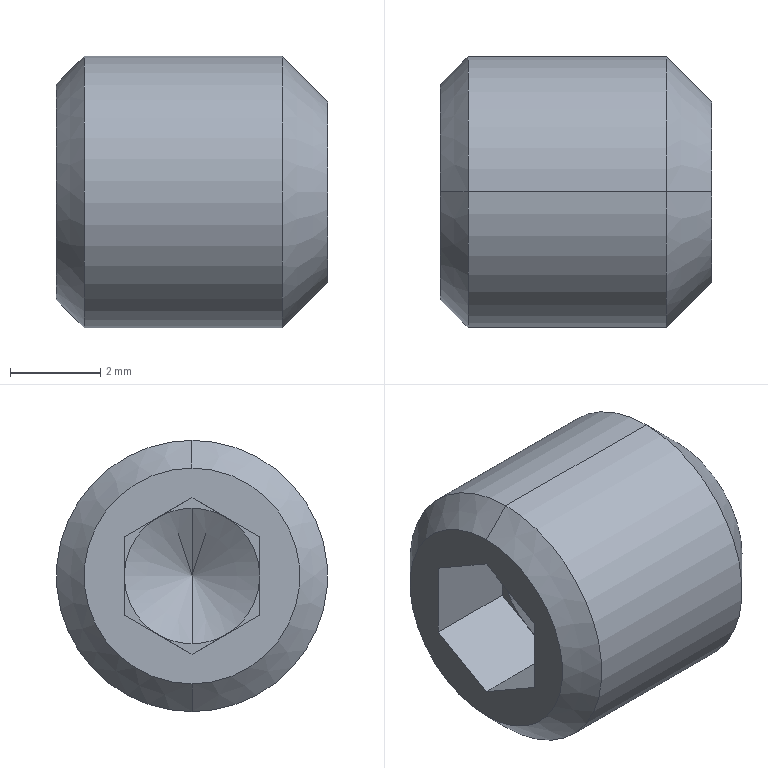Part | SolidWorks | features BaseBody 1 | 1 solid | 22 faces | box 6 x 6 x 6 mm | volume 140.334 mm3 | plane 14 | cone 6 | cylinder 2 | commonest cylinder face diameters 6 x2
STEP:
#1=CARTESIAN_POINT('',(-1.,0.,3.));
#2=VERTEX_POINT('',#1);
#3=CARTESIAN_POINT('',(-1.,0.,-3.));
#4=VERTEX_POINT('',#3);
#5=CARTESIAN_POINT('',(-1.,0.,0.));
#6=DIRECTION('',(-1.,0.,0.));
#7=DIRECTION('',(0.,0.,1.));
#8=AXIS2_PLACEMENT_3D('',#5,#6,#7);
#9=CIRCLE('',#8,3.);
#10=EDGE_CURVE('',#2,#4,#9,.T.);
#11=ORIENTED_EDGE('',*,*,#10,.T.);
#12=CARTESIAN_POINT('',(-5.386,0.,-3.));
#13=VERTEX_POINT('',#12);
#14=CARTESIAN_POINT('',(0.,0.,-3.));
#15=DIRECTION('',(-1.,0.,0.));
#16=VECTOR('',#15,1000.);
#17=LINE('',#14,#16);
#18=EDGE_CURVE('',#4,#13,#17,.T.);
#19=ORIENTED_EDGE('',*,*,#18,.T.);
#20=CARTESIAN_POINT('',(-5.386,0.,3.));
#21=VERTEX_POINT('',#20);
#22=CARTESIAN_POINT('',(-5.386,0.,0.));
#23=DIRECTION('',(1.,0.,0.));
#24=DIRECTION('',(0.,0.,1.));
#25=AXIS2_PLACEMENT_3D('',#22,#23,#24);
#26=CIRCLE('',#25,3.);
#27=EDGE_CURVE('',#13,#21,#26,.T.);
#28=ORIENTED_EDGE('',*,*,#27,.T.);
#29=CARTESIAN_POINT('',(0.,0.,3.));
#30=DIRECTION('',(-1.,0.,0.));
#31=VECTOR('',#30,1000.);
#32=LINE('',#29,#31);
#33=EDGE_CURVE('',#2,#21,#32,.T.);
#34=ORIENTED_EDGE('',*,*,#33,.F.);
#35=EDGE_LOOP('',(#11,#19,#28,#34));
#36=FACE_OUTER_BOUND('',#35,.T.);
#37=CARTESIAN_POINT('',(0.,0.,0.));
#38=DIRECTION('',(-1.,0.,0.));
#39=DIRECTION('',(0.,0.,1.));
#40=AXIS2_PLACEMENT_3D('',#37,#38,#39);
#41=CYLINDRICAL_SURFACE('',#40,3.);
#42=ADVANCED_FACE('',(#36),#41,.T.);
#43=CARTESIAN_POINT('',(-6.,0.,-2.387));
#44=VERTEX_POINT('',#43);
#45=CARTESIAN_POINT('',(-6.,0.,2.387));
#46=VERTEX_POINT('',#45);
#47=CARTESIAN_POINT('',(-6.,0.,0.));
#48=DIRECTION('',(1.,0.,0.));
#49=DIRECTION('',(0.,0.,-1.));
#50=AXIS2_PLACEMENT_3D('',#47,#48,#49);
#51=CIRCLE('',#50,2.387);
#52=EDGE_CURVE('',#44,#46,#51,.T.);
#53=ORIENTED_EDGE('',*,*,#52,.T.);
#54=CARTESIAN_POINT('',(-5.386,0.,3.));
#55=DIRECTION('',(0.7071,0.,0.7071));
#56=VECTOR('',#55,1000.);
#57=LINE('',#54,#56);
#58=EDGE_CURVE('',#46,#21,#57,.T.);
#59=ORIENTED_EDGE('',*,*,#58,.T.);
#60=ORIENTED_EDGE('',*,*,#27,.F.);
#61=CARTESIAN_POINT('',(-5.386,0.,-3.));
#62=DIRECTION('',(0.7071,0.,-0.7071));
#63=VECTOR('',#62,1000.);
#64=LINE('',#61,#63);
#65=EDGE_CURVE('',#44,#13,#64,.T.);
#66=ORIENTED_EDGE('',*,*,#65,.F.);
#67=EDGE_LOOP('',(#53,#59,#60,#66));
#68=FACE_OUTER_BOUND('',#67,.T.);
#69=CARTESIAN_POINT('',(-5.386,0.,0.));
#70=DIRECTION('',(1.,0.,0.));
#71=DIRECTION('',(0.,0.,-1.));
#72=AXIS2_PLACEMENT_3D('',#69,#70,#71);
#73=CONICAL_SURFACE('',#72,3.,0.7854);
#74=ADVANCED_FACE('',(#68),#73,.T.);
#75=CARTESIAN_POINT('',(0.,0.,2.));
#76=VERTEX_POINT('',#75);
#77=CARTESIAN_POINT('',(0.,0.,-2.));
#78=VERTEX_POINT('',#77);
#79=CARTESIAN_POINT('',(0.,0.,0.));
#80=DIRECTION('',(-1.,0.,0.));
#81=DIRECTION('',(0.,0.,1.));
#82=AXIS2_PLACEMENT_3D('',#79,#80,#81);
#83=CIRCLE('',#82,2.);
#84=EDGE_CURVE('',#76,#78,#83,.T.);
#85=ORIENTED_EDGE('',*,*,#84,.T.);
#86=CARTESIAN_POINT('',(-1.,0.,-3.));
#87=DIRECTION('',(-0.7071,0.,-0.7071));
#88=VECTOR('',#87,1000.);
#89=LINE('',#86,#88);
#90=EDGE_CURVE('',#78,#4,#89,.T.);
#91=ORIENTED_EDGE('',*,*,#90,.T.);
#92=ORIENTED_EDGE('',*,*,#10,.F.);
#93=CARTESIAN_POINT('',(-1.,0.,3.));
#94=DIRECTION('',(-0.7071,0.,0.7071));
#95=VECTOR('',#94,1000.);
#96=LINE('',#93,#95);
#97=EDGE_CURVE('',#76,#2,#96,.T.);
#98=ORIENTED_EDGE('',*,*,#97,.F.);
#99=EDGE_LOOP('',(#85,#91,#92,#98));
#100=FACE_OUTER_BOUND('',#99,.T.);
#101=CARTESIAN_POINT('',(-1.,0.,0.));
#102=DIRECTION('',(-1.,0.,0.));
#103=DIRECTION('',(0.,0.,1.));
#104=AXIS2_PLACEMENT_3D('',#101,#102,#103);
#105=CONICAL_SURFACE('',#104,3.,0.7854);
#106=ADVANCED_FACE('',(#100),#105,.T.);
#107=CARTESIAN_POINT('',(-3.134,0.,0.));
#108=VERTEX_POINT('',#107);
#109=CARTESIAN_POINT('',(-4.,0.,1.5));
#110=VERTEX_POINT('',#109);
#111=CARTESIAN_POINT('',(-4.,0.,1.5));
#112=DIRECTION('',(-0.5,0.,0.866));
#113=VECTOR('',#112,1000.);
#114=LINE('',#111,#113);
#115=EDGE_CURVE('',#108,#110,#114,.T.);
#116=ORIENTED_EDGE('',*,*,#115,.F.);
#117=CARTESIAN_POINT('',(-4.,0.,-1.5));
#118=VERTEX_POINT('',#117);
#119=CARTESIAN_POINT('',(-4.,0.,-1.5));
#120=DIRECTION('',(-0.5,0.,-0.866));
#121=VECTOR('',#120,1000.);
#122=LINE('',#119,#121);
#123=EDGE_CURVE('',#108,#118,#122,.T.);
#124=ORIENTED_EDGE('',*,*,#123,.T.);
#125=CARTESIAN_POINT('',(-4.,-0.75,-1.299));
#126=VERTEX_POINT('',#125);
#127=CARTESIAN_POINT('',(-4.,0.,0.));
#128=DIRECTION('',(1.,0.,0.));
#129=DIRECTION('',(0.,0.,1.));
#130=AXIS2_PLACEMENT_3D('',#127,#128,#129);
#131=CIRCLE('',#130,1.5);
#132=EDGE_CURVE('',#126,#118,#131,.T.);
#133=ORIENTED_EDGE('',*,*,#132,.F.);
#134=CARTESIAN_POINT('',(-4.,-1.5,0.));
#135=VERTEX_POINT('',#134);
#136=CARTESIAN_POINT('',(-4.,0.,0.));
#137=DIRECTION('',(1.,0.,0.));
#138=DIRECTION('',(0.,0.,1.));
#139=AXIS2_PLACEMENT_3D('',#136,#137,#138);
#140=CIRCLE('',#139,1.5);
#141=EDGE_CURVE('',#135,#126,#140,.T.);
#142=ORIENTED_EDGE('',*,*,#141,.F.);
#143=CARTESIAN_POINT('',(-4.,-0.75,1.299));
#144=VERTEX_POINT('',#143);
#145=CARTESIAN_POINT('',(-4.,0.,0.));
#146=DIRECTION('',(1.,0.,0.));
#147=DIRECTION('',(0.,0.,1.));
#148=AXIS2_PLACEMENT_3D('',#145,#146,#147);
#149=CIRCLE('',#148,1.5);
#150=EDGE_CURVE('',#144,#135,#149,.T.);
#151=ORIENTED_EDGE('',*,*,#150,.F.);
#152=CARTESIAN_POINT('',(-4.,0.,0.));
#153=DIRECTION('',(1.,0.,0.));
#154=DIRECTION('',(0.,0.,1.));
#155=AXIS2_PLACEMENT_3D('',#152,#153,#154);
#156=CIRCLE('',#155,1.5);
#157=EDGE_CURVE('',#110,#144,#156,.T.);
#158=ORIENTED_EDGE('',*,*,#157,.F.);
#159=EDGE_LOOP('',(#116,#124,#133,#142,#151,#158));
#160=FACE_OUTER_BOUND('',#159,.T.);
#161=CARTESIAN_POINT('',(-4.,0.,0.));
#162=DIRECTION('',(-1.,0.,0.));
#163=DIRECTION('',(0.,0.,1.));
#164=AXIS2_PLACEMENT_3D('',#161,#162,#163);
#165=CONICAL_SURFACE('',#164,1.5,1.047);
#166=ADVANCED_FACE('',(#160),#165,.F.);
#167=ORIENTED_EDGE('',*,*,#18,.F.);
#168=CARTESIAN_POINT('',(-1.,0.,0.));
#169=DIRECTION('',(-1.,0.,0.));
#170=DIRECTION('',(0.,0.,1.));
#171=AXIS2_PLACEMENT_3D('',#168,#169,#170);
#172=CIRCLE('',#171,3.);
#173=EDGE_CURVE('',#4,#2,#172,.T.);
#174=ORIENTED_EDGE('',*,*,#173,.T.);
#175=ORIENTED_EDGE('',*,*,#33,.T.);
#176=CARTESIAN_POINT('',(-5.386,0.,0.));
#177=DIRECTION('',(1.,0.,0.));
#178=DIRECTION('',(0.,0.,1.));
#179=AXIS2_PLACEMENT_3D('',#176,#177,#178);
#180=CIRCLE('',#179,3.);
#181=EDGE_CURVE('',#21,#13,#180,.T.);
#182=ORIENTED_EDGE('',*,*,#181,.T.);
#183=EDGE_LOOP('',(#167,#174,#175,#182));
#184=FACE_OUTER_BOUND('',#183,.T.);
#185=CARTESIAN_POINT('',(0.,0.,0.));
#186=DIRECTION('',(-1.,0.,0.));
#187=DIRECTION('',(0.,0.,1.));
#188=AXIS2_PLACEMENT_3D('',#185,#186,#187);
#189=CYLINDRICAL_SURFACE('',#188,3.);
#190=ADVANCED_FACE('',(#184),#189,.T.);
#191=ORIENTED_EDGE('',*,*,#58,.F.);
#192=CARTESIAN_POINT('',(-6.,0.,0.));
#193=DIRECTION('',(1.,0.,0.));
#194=DIRECTION('',(0.,0.,-1.));
#195=AXIS2_PLACEMENT_3D('',#192,#193,#194);
#196=CIRCLE('',#195,2.387);
#197=EDGE_CURVE('',#46,#44,#196,.T.);
#198=ORIENTED_EDGE('',*,*,#197,.T.);
#199=ORIENTED_EDGE('',*,*,#65,.T.);
#200=ORIENTED_EDGE('',*,*,#181,.F.);
#201=EDGE_LOOP('',(#191,#198,#199,#200));
#202=FACE_OUTER_BOUND('',#201,.T.);
#203=CARTESIAN_POINT('',(-5.386,0.,0.));
#204=DIRECTION('',(1.,0.,0.));
#205=DIRECTION('',(0.,0.,-1.));
#206=AXIS2_PLACEMENT_3D('',#203,#204,#205);
#207=CONICAL_SURFACE('',#206,3.,0.7854);
#208=ADVANCED_FACE('',(#202),#207,.T.);
#209=ORIENTED_EDGE('',*,*,#90,.F.);
#210=CARTESIAN_POINT('',(0.,0.,0.));
#211=DIRECTION('',(-1.,0.,0.));
#212=DIRECTION('',(0.,0.,1.));
#213=AXIS2_PLACEMENT_3D('',#210,#211,#212);
#214=CIRCLE('',#213,2.);
#215=EDGE_CURVE('',#78,#76,#214,.T.);
#216=ORIENTED_EDGE('',*,*,#215,.T.);
#217=ORIENTED_EDGE('',*,*,#97,.T.);
#218=ORIENTED_EDGE('',*,*,#173,.F.);
#219=EDGE_LOOP('',(#209,#216,#217,#218));
#220=FACE_OUTER_BOUND('',#219,.T.);
#221=CARTESIAN_POINT('',(-1.,0.,0.));
#222=DIRECTION('',(-1.,0.,0.));
#223=DIRECTION('',(0.,0.,1.));
#224=AXIS2_PLACEMENT_3D('',#221,#222,#223);
#225=CONICAL_SURFACE('',#224,3.,0.7854);
#226=ADVANCED_FACE('',(#220),#225,.T.);
#227=CARTESIAN_POINT('',(-6.,0.,1.732));
#228=VERTEX_POINT('',#227);
#229=CARTESIAN_POINT('',(-6.,-1.5,0.866));
#230=VERTEX_POINT('',#229);
#231=CARTESIAN_POINT('',(-6.,-1.5,0.866));
#232=DIRECTION('',(0.,-0.866,-0.5));
#233=VECTOR('',#232,1000.);
#234=LINE('',#231,#233);
#235=EDGE_CURVE('',#228,#230,#234,.T.);
#236=ORIENTED_EDGE('',*,*,#235,.T.);
#237=CARTESIAN_POINT('',(-6.,-1.5,-0.866));
#238=VERTEX_POINT('',#237);
#239=CARTESIAN_POINT('',(-6.,-1.5,-0.866));
#240=DIRECTION('',(0.,0.,-1.));
#241=VECTOR('',#240,1000.);
#242=LINE('',#239,#241);
#243=EDGE_CURVE('',#230,#238,#242,.T.);
#244=ORIENTED_EDGE('',*,*,#243,.T.);
#245=CARTESIAN_POINT('',(-6.,0.,-1.732));
#246=VERTEX_POINT('',#245);
#247=CARTESIAN_POINT('',(-6.,0.,-1.732));
#248=DIRECTION('',(0.,0.866,-0.5));
#249=VECTOR('',#248,1000.);
#250=LINE('',#247,#249);
#251=EDGE_CURVE('',#238,#246,#250,.T.);
#252=ORIENTED_EDGE('',*,*,#251,.T.);
#253=CARTESIAN_POINT('',(-6.,1.5,-0.866));
#254=VERTEX_POINT('',#253);
#255=CARTESIAN_POINT('',(-6.,1.5,-0.866));
#256=DIRECTION('',(0.,0.866,0.5));
#257=VECTOR('',#256,1000.);
#258=LINE('',#255,#257);
#259=EDGE_CURVE('',#246,#254,#258,.T.);
#260=ORIENTED_EDGE('',*,*,#259,.T.);
#261=CARTESIAN_POINT('',(-6.,1.5,0.866));
#262=VERTEX_POINT('',#261);
#263=CARTESIAN_POINT('',(-6.,1.5,0.866));
#264=DIRECTION('',(0.,0.,1.));
#265=VECTOR('',#264,1000.);
#266=LINE('',#263,#265);
#267=EDGE_CURVE('',#254,#262,#266,.T.);
#268=ORIENTED_EDGE('',*,*,#267,.T.);
#269=CARTESIAN_POINT('',(-6.,0.,1.732));
#270=DIRECTION('',(0.,0.866,-0.5));
#271=VECTOR('',#270,1000.);
#272=LINE('',#269,#271);
#273=EDGE_CURVE('',#228,#262,#272,.T.);
#274=ORIENTED_EDGE('',*,*,#273,.F.);
#275=EDGE_LOOP('',(#236,#244,#252,#260,#268,#274));
#276=FACE_BOUND('',#275,.T.);
#277=ORIENTED_EDGE('',*,*,#52,.F.);
#278=ORIENTED_EDGE('',*,*,#197,.F.);
#279=EDGE_LOOP('',(#277,#278));
#280=FACE_OUTER_BOUND('',#279,.T.);
#281=CARTESIAN_POINT('',(-6.,0.,0.));
#282=DIRECTION('',(1.,0.,0.));
#283=DIRECTION('',(0.,0.,-1.));
#284=AXIS2_PLACEMENT_3D('',#281,#282,#283);
#285=PLANE('',#284);
#286=ADVANCED_FACE('',(#276,#280),#285,.F.);
#287=ORIENTED_EDGE('',*,*,#84,.F.);
#288=ORIENTED_EDGE('',*,*,#215,.F.);
#289=EDGE_LOOP('',(#287,#288));
#290=FACE_OUTER_BOUND('',#289,.T.);
#291=CARTESIAN_POINT('',(0.,2.,0.));
#292=DIRECTION('',(-1.,0.,0.));
#293=DIRECTION('',(0.,0.,1.));
#294=AXIS2_PLACEMENT_3D('',#291,#292,#293);
#295=PLANE('',#294);
#296=ADVANCED_FACE('',(#290),#295,.F.);
#297=CARTESIAN_POINT('',(-4.,1.5,0.866));
#298=VERTEX_POINT('',#297);
#299=CARTESIAN_POINT('',(-4.,1.5,0.866));
#300=DIRECTION('',(-1.,0.,0.));
#301=VECTOR('',#300,1000.);
#302=LINE('',#299,#301);
#303=EDGE_CURVE('',#298,#262,#302,.T.);
#304=ORIENTED_EDGE('',*,*,#303,.F.);
#305=CARTESIAN_POINT('',(-4.,0.75,1.299));
#306=VERTEX_POINT('',#305);
#307=CARTESIAN_POINT('',(-4.,0.,1.732));
#308=DIRECTION('',(0.,0.866,-0.5));
#309=VECTOR('',#308,1000.);
#310=LINE('',#307,#309);
#311=EDGE_CURVE('',#306,#298,#310,.T.);
#312=ORIENTED_EDGE('',*,*,#311,.F.);
#313=CARTESIAN_POINT('',(-4.,0.,1.732));
#314=VERTEX_POINT('',#313);
#315=CARTESIAN_POINT('',(-4.,0.,1.732));
#316=DIRECTION('',(0.,0.866,-0.5));
#317=VECTOR('',#316,1000.);
#318=LINE('',#315,#317);
#319=EDGE_CURVE('',#314,#306,#318,.T.);
#320=ORIENTED_EDGE('',*,*,#319,.F.);
#321=CARTESIAN_POINT('',(-4.,0.,1.732));
#322=DIRECTION('',(1.,0.,0.));
#323=VECTOR('',#322,1000.);
#324=LINE('',#321,#323);
#325=EDGE_CURVE('',#228,#314,#324,.T.);
#326=ORIENTED_EDGE('',*,*,#325,.F.);
#327=ORIENTED_EDGE('',*,*,#273,.T.);
#328=EDGE_LOOP('',(#304,#312,#320,#326,#327));
#329=FACE_OUTER_BOUND('',#328,.T.);
#330=CARTESIAN_POINT('',(-4.,0.,1.732));
#331=DIRECTION('',(0.,0.5,0.866));
#332=DIRECTION('',(0.,-0.866,0.5));
#333=AXIS2_PLACEMENT_3D('',#330,#331,#332);
#334=PLANE('',#333);
#335=ADVANCED_FACE('',(#329),#334,.F.);
#336=ORIENTED_EDGE('',*,*,#267,.F.);
#337=CARTESIAN_POINT('',(-4.,1.5,-0.866));
#338=VERTEX_POINT('',#337);
#339=CARTESIAN_POINT('',(-4.,1.5,-0.866));
#340=DIRECTION('',(-1.,0.,0.));
#341=VECTOR('',#340,1000.);
#342=LINE('',#339,#341);
#343=EDGE_CURVE('',#338,#254,#342,.T.);
#344=ORIENTED_EDGE('',*,*,#343,.F.);
#345=CARTESIAN_POINT('',(-4.,1.5,0.));
#346=VERTEX_POINT('',#345);
#347=CARTESIAN_POINT('',(-4.,1.5,0.866));
#348=DIRECTION('',(0.,0.,-1.));
#349=VECTOR('',#348,1000.);
#350=LINE('',#347,#349);
#351=EDGE_CURVE('',#346,#338,#350,.T.);
#352=ORIENTED_EDGE('',*,*,#351,.F.);
#353=CARTESIAN_POINT('',(-4.,1.5,0.866));
#354=DIRECTION('',(0.,0.,-1.));
#355=VECTOR('',#354,1000.);
#356=LINE('',#353,#355);
#357=EDGE_CURVE('',#298,#346,#356,.T.);
#358=ORIENTED_EDGE('',*,*,#357,.F.);
#359=ORIENTED_EDGE('',*,*,#303,.T.);
#360=EDGE_LOOP('',(#336,#344,#352,#358,#359));
#361=FACE_OUTER_BOUND('',#360,.T.);
#362=CARTESIAN_POINT('',(-4.,1.5,0.866));
#363=DIRECTION('',(0.,1.,0.));
#364=DIRECTION('',(0.,0.,1.));
#365=AXIS2_PLACEMENT_3D('',#362,#363,#364);
#366=PLANE('',#365);
#367=ADVANCED_FACE('',(#361),#366,.F.);
#368=CARTESIAN_POINT('',(-4.,0.,0.));
#369=DIRECTION('',(1.,0.,0.));
#370=DIRECTION('',(0.,0.,1.));
#371=AXIS2_PLACEMENT_3D('',#368,#369,#370);
#372=CIRCLE('',#371,1.5);
#373=EDGE_CURVE('',#346,#306,#372,.T.);
#374=ORIENTED_EDGE('',*,*,#373,.T.);
#375=ORIENTED_EDGE('',*,*,#311,.T.);
#376=ORIENTED_EDGE('',*,*,#357,.T.);
#377=EDGE_LOOP('',(#374,#375,#376));
#378=FACE_OUTER_BOUND('',#377,.T.);
#379=CARTESIAN_POINT('',(-4.,0.,0.));
#380=DIRECTION('',(-1.,0.,0.));
#381=DIRECTION('',(0.,0.,1.));
#382=AXIS2_PLACEMENT_3D('',#379,#380,#381);
#383=PLANE('',#382);
#384=ADVANCED_FACE('',(#378),#383,.T.);
#385=CARTESIAN_POINT('',(-4.,0.,0.));
#386=DIRECTION('',(1.,0.,0.));
#387=DIRECTION('',(0.,0.,1.));
#388=AXIS2_PLACEMENT_3D('',#385,#386,#387);
#389=CIRCLE('',#388,1.5);
#390=EDGE_CURVE('',#306,#110,#389,.T.);
#391=ORIENTED_EDGE('',*,*,#390,.T.);
#392=ORIENTED_EDGE('',*,*,#157,.T.);
#393=CARTESIAN_POINT('',(-4.,-0.75,1.299));
#394=DIRECTION('',(0.,0.866,0.5));
#395=VECTOR('',#394,1000.);
#396=LINE('',#393,#395);
#397=EDGE_CURVE('',#144,#314,#396,.T.);
#398=ORIENTED_EDGE('',*,*,#397,.T.);
#399=ORIENTED_EDGE('',*,*,#319,.T.);
#400=EDGE_LOOP('',(#391,#392,#398,#399));
#401=FACE_OUTER_BOUND('',#400,.T.);
#402=CARTESIAN_POINT('',(-4.,0.,0.));
#403=DIRECTION('',(-1.,0.,0.));
#404=DIRECTION('',(0.,0.,1.));
#405=AXIS2_PLACEMENT_3D('',#402,#403,#404);
#406=PLANE('',#405);
#407=ADVANCED_FACE('',(#401),#406,.T.);
#408=ORIENTED_EDGE('',*,*,#325,.T.);
#409=ORIENTED_EDGE('',*,*,#397,.F.);
#410=CARTESIAN_POINT('',(-4.,-1.5,0.866));
#411=VERTEX_POINT('',#410);
#412=CARTESIAN_POINT('',(-4.,-1.5,0.866));
#413=DIRECTION('',(0.,0.866,0.5));
#414=VECTOR('',#413,1000.);
#415=LINE('',#412,#414);
#416=EDGE_CURVE('',#411,#144,#415,.T.);
#417=ORIENTED_EDGE('',*,*,#416,.F.);
#418=CARTESIAN_POINT('',(-4.,-1.5,0.866));
#419=DIRECTION('',(1.,0.,0.));
#420=VECTOR('',#419,1000.);
#421=LINE('',#418,#420);
#422=EDGE_CURVE('',#230,#411,#421,.T.);
#423=ORIENTED_EDGE('',*,*,#422,.F.);
#424=ORIENTED_EDGE('',*,*,#235,.F.);
#425=EDGE_LOOP('',(#408,#409,#417,#423,#424));
#426=FACE_OUTER_BOUND('',#425,.T.);
#427=CARTESIAN_POINT('',(-4.,-1.5,0.866));
#428=DIRECTION('',(0.,-0.5,0.866));
#429=DIRECTION('',(0.,-0.866,-0.5));
#430=AXIS2_PLACEMENT_3D('',#427,#428,#429);
#431=PLANE('',#430);
#432=ADVANCED_FACE('',(#426),#431,.F.);
#433=CARTESIAN_POINT('',(-4.,0.,-1.732));
#434=VERTEX_POINT('',#433);
#435=CARTESIAN_POINT('',(-4.,0.,-1.732));
#436=DIRECTION('',(-1.,0.,0.));
#437=VECTOR('',#436,1000.);
#438=LINE('',#435,#437);
#439=EDGE_CURVE('',#434,#246,#438,.T.);
#440=ORIENTED_EDGE('',*,*,#439,.F.);
#441=CARTESIAN_POINT('',(-4.,0.75,-1.299));
#442=VERTEX_POINT('',#441);
#443=CARTESIAN_POINT('',(-4.,1.5,-0.866));
#444=DIRECTION('',(0.,-0.866,-0.5));
#445=VECTOR('',#444,1000.);
#446=LINE('',#443,#445);
#447=EDGE_CURVE('',#442,#434,#446,.T.);
#448=ORIENTED_EDGE('',*,*,#447,.F.);
#449=CARTESIAN_POINT('',(-4.,1.5,-0.866));
#450=DIRECTION('',(0.,-0.866,-0.5));
#451=VECTOR('',#450,1000.);
#452=LINE('',#449,#451);
#453=EDGE_CURVE('',#338,#442,#452,.T.);
#454=ORIENTED_EDGE('',*,*,#453,.F.);
#455=ORIENTED_EDGE('',*,*,#343,.T.);
#456=ORIENTED_EDGE('',*,*,#259,.F.);
#457=EDGE_LOOP('',(#440,#448,#454,#455,#456));
#458=FACE_OUTER_BOUND('',#457,.T.);
#459=CARTESIAN_POINT('',(-4.,1.5,-0.866));
#460=DIRECTION('',(0.,0.5,-0.866));
#461=DIRECTION('',(0.,0.866,0.5));
#462=AXIS2_PLACEMENT_3D('',#459,#460,#461);
#463=PLANE('',#462);
#464=ADVANCED_FACE('',(#458),#463,.F.);
#465=CARTESIAN_POINT('',(-4.,0.,0.));
#466=DIRECTION('',(1.,0.,0.));
#467=DIRECTION('',(0.,0.,1.));
#468=AXIS2_PLACEMENT_3D('',#465,#466,#467);
#469=CIRCLE('',#468,1.5);
#470=EDGE_CURVE('',#442,#346,#469,.T.);
#471=ORIENTED_EDGE('',*,*,#470,.T.);
#472=ORIENTED_EDGE('',*,*,#351,.T.);
#473=ORIENTED_EDGE('',*,*,#453,.T.);
#474=EDGE_LOOP('',(#471,#472,#473));
#475=FACE_OUTER_BOUND('',#474,.T.);
#476=CARTESIAN_POINT('',(-4.,0.,0.));
#477=DIRECTION('',(-1.,0.,0.));
#478=DIRECTION('',(0.,0.,1.));
#479=AXIS2_PLACEMENT_3D('',#476,#477,#478);
#480=PLANE('',#479);
#481=ADVANCED_FACE('',(#475),#480,.T.);
#482=ORIENTED_EDGE('',*,*,#123,.F.);
#483=ORIENTED_EDGE('',*,*,#115,.T.);
#484=ORIENTED_EDGE('',*,*,#390,.F.);
#485=ORIENTED_EDGE('',*,*,#373,.F.);
#486=ORIENTED_EDGE('',*,*,#470,.F.);
#487=CARTESIAN_POINT('',(-4.,0.,0.));
#488=DIRECTION('',(1.,0.,0.));
#489=DIRECTION('',(0.,0.,1.));
#490=AXIS2_PLACEMENT_3D('',#487,#488,#489);
#491=CIRCLE('',#490,1.5);
#492=EDGE_CURVE('',#118,#442,#491,.T.);
#493=ORIENTED_EDGE('',*,*,#492,.F.);
#494=EDGE_LOOP('',(#482,#483,#484,#485,#486,#493));
#495=FACE_OUTER_BOUND('',#494,.T.);
#496=CARTESIAN_POINT('',(-4.,0.,0.));
#497=DIRECTION('',(-1.,0.,0.));
#498=DIRECTION('',(0.,0.,1.));
#499=AXIS2_PLACEMENT_3D('',#496,#497,#498);
#500=CONICAL_SURFACE('',#499,1.5,1.047);
#501=ADVANCED_FACE('',(#495),#500,.F.);
#502=ORIENTED_EDGE('',*,*,#150,.T.);
#503=CARTESIAN_POINT('',(-4.,-1.5,0.));
#504=DIRECTION('',(0.,0.,1.));
#505=VECTOR('',#504,1000.);
#506=LINE('',#503,#505);
#507=EDGE_CURVE('',#135,#411,#506,.T.);
#508=ORIENTED_EDGE('',*,*,#507,.T.);
#509=ORIENTED_EDGE('',*,*,#416,.T.);
#510=EDGE_LOOP('',(#502,#508,#509));
#511=FACE_OUTER_BOUND('',#510,.T.);
#512=CARTESIAN_POINT('',(-4.,0.,0.));
#513=DIRECTION('',(-1.,0.,0.));
#514=DIRECTION('',(0.,0.,1.));
#515=AXIS2_PLACEMENT_3D('',#512,#513,#514);
#516=PLANE('',#515);
#517=ADVANCED_FACE('',(#511),#516,.T.);
#518=ORIENTED_EDGE('',*,*,#422,.T.);
#519=ORIENTED_EDGE('',*,*,#507,.F.);
#520=CARTESIAN_POINT('',(-4.,-1.5,-0.866));
#521=VERTEX_POINT('',#520);
#522=CARTESIAN_POINT('',(-4.,-1.5,-0.866));
#523=DIRECTION('',(0.,0.,1.));
#524=VECTOR('',#523,1000.);
#525=LINE('',#522,#524);
#526=EDGE_CURVE('',#521,#135,#525,.T.);
#527=ORIENTED_EDGE('',*,*,#526,.F.);
#528=CARTESIAN_POINT('',(-4.,-1.5,-0.866));
#529=DIRECTION('',(1.,0.,0.));
#530=VECTOR('',#529,1000.);
#531=LINE('',#528,#530);
#532=EDGE_CURVE('',#238,#521,#531,.T.);
#533=ORIENTED_EDGE('',*,*,#532,.F.);
#534=ORIENTED_EDGE('',*,*,#243,.F.);
#535=EDGE_LOOP('',(#518,#519,#527,#533,#534));
#536=FACE_OUTER_BOUND('',#535,.T.);
#537=CARTESIAN_POINT('',(-4.,-1.5,-0.866));
#538=DIRECTION('',(0.,-1.,0.));
#539=DIRECTION('',(0.,0.,-1.));
#540=AXIS2_PLACEMENT_3D('',#537,#538,#539);
#541=PLANE('',#540);
#542=ADVANCED_FACE('',(#536),#541,.F.);
#543=ORIENTED_EDGE('',*,*,#532,.T.);
#544=CARTESIAN_POINT('',(-4.,0.,-1.732));
#545=DIRECTION('',(0.,-0.866,0.5));
#546=VECTOR('',#545,1000.);
#547=LINE('',#544,#546);
#548=EDGE_CURVE('',#126,#521,#547,.T.);
#549=ORIENTED_EDGE('',*,*,#548,.F.);
#550=CARTESIAN_POINT('',(-4.,0.,-1.732));
#551=DIRECTION('',(0.,-0.866,0.5));
#552=VECTOR('',#551,1000.);
#553=LINE('',#550,#552);
#554=EDGE_CURVE('',#434,#126,#553,.T.);
#555=ORIENTED_EDGE('',*,*,#554,.F.);
#556=ORIENTED_EDGE('',*,*,#439,.T.);
#557=ORIENTED_EDGE('',*,*,#251,.F.);
#558=EDGE_LOOP('',(#543,#549,#555,#556,#557));
#559=FACE_OUTER_BOUND('',#558,.T.);
#560=CARTESIAN_POINT('',(-4.,0.,-1.732));
#561=DIRECTION('',(0.,-0.5,-0.866));
#562=DIRECTION('',(0.,0.866,-0.5));
#563=AXIS2_PLACEMENT_3D('',#560,#561,#562);
#564=PLANE('',#563);
#565=ADVANCED_FACE('',(#559),#564,.F.);
#566=ORIENTED_EDGE('',*,*,#132,.T.);
#567=ORIENTED_EDGE('',*,*,#492,.T.);
#568=ORIENTED_EDGE('',*,*,#447,.T.);
#569=ORIENTED_EDGE('',*,*,#554,.T.);
#570=EDGE_LOOP('',(#566,#567,#568,#569));
#571=FACE_OUTER_BOUND('',#570,.T.);
#572=CARTESIAN_POINT('',(-4.,0.,0.));
#573=DIRECTION('',(-1.,0.,0.));
#574=DIRECTION('',(0.,0.,1.));
#575=AXIS2_PLACEMENT_3D('',#572,#573,#574);
#576=PLANE('',#575);
#577=ADVANCED_FACE('',(#571),#576,.T.);
#578=ORIENTED_EDGE('',*,*,#141,.T.);
#579=ORIENTED_EDGE('',*,*,#548,.T.);
#580=ORIENTED_EDGE('',*,*,#526,.T.);
#581=EDGE_LOOP('',(#578,#579,#580));
#582=FACE_OUTER_BOUND('',#581,.T.);
#583=CARTESIAN_POINT('',(-4.,0.,0.));
#584=DIRECTION('',(-1.,0.,0.));
#585=DIRECTION('',(0.,0.,1.));
#586=AXIS2_PLACEMENT_3D('',#583,#584,#585);
#587=PLANE('',#586);
#588=ADVANCED_FACE('',(#582),#587,.T.);
#589=CLOSED_SHELL('',(#42,#74,#106,#166,#190,#208,#226,#286,#296,#335,#367,#384,#407,#432,#464,#481,#501,#517,#542,#565,#577,#588));
#590=MANIFOLD_SOLID_BREP('',#589);
#591=CARTESIAN_POINT('',(0.,0.,0.));
#592=DIRECTION('',(0.,0.,1.));
#593=DIRECTION('',(1.,0.,0.));
#594=AXIS2_PLACEMENT_3D('',#591,#592,#593);
#595=(LENGTH_UNIT()NAMED_UNIT(*)SI_UNIT(.MILLI.,.METRE.));
#596=UNCERTAINTY_MEASURE_WITH_UNIT(LENGTH_MEASURE(0.00001),#595,'','');
#597=(NAMED_UNIT(*)PLANE_ANGLE_UNIT()SI_UNIT($,.RADIAN.));
#598=(NAMED_UNIT(*)SI_UNIT($,.STERADIAN.)SOLID_ANGLE_UNIT());
#599=(GEOMETRIC_REPRESENTATION_CONTEXT(3)GLOBAL_UNCERTAINTY_ASSIGNED_CONTEXT((#596))GLOBAL_UNIT_ASSIGNED_CONTEXT((#595,#597,#598))REPRESENTATION_CONTEXT('',''));
#600=ADVANCED_BREP_SHAPE_REPRESENTATION('',(#590,#594),#599);